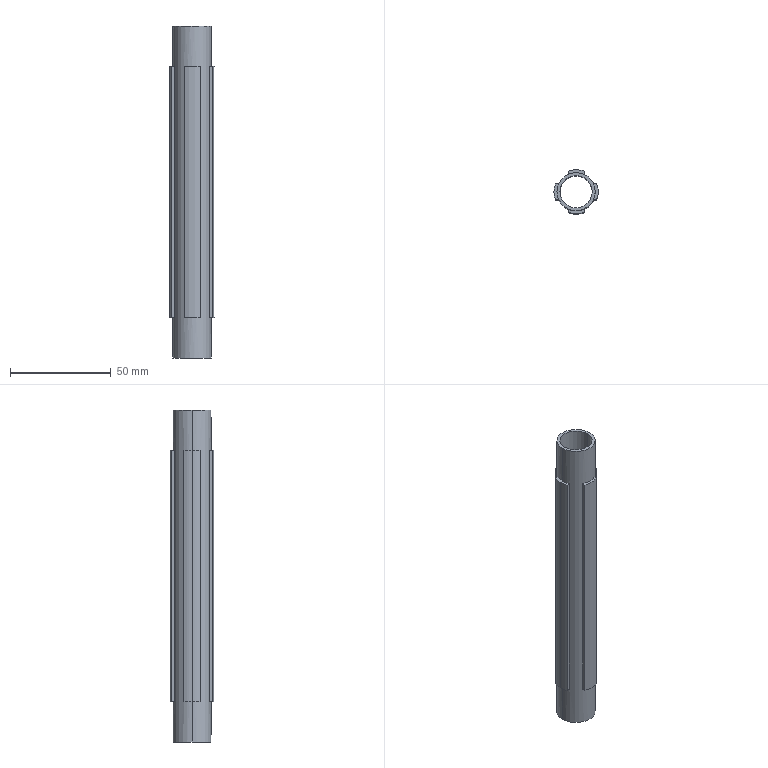Part | SolidWorks | features Extrusion 1, ICE 1 | 1 solid | 27 faces | box 22 x 22 x 165 mm | volume 19772 mm3 | plane 18 | cylinder 9 | commonest cylinder face diameters 22 x5 16 x2 19 x2
STEP:
#1=CARTESIAN_POINT('',(-8.,0.,145.));
#2=VERTEX_POINT('',#1);
#3=CARTESIAN_POINT('',(8.,0.,145.));
#4=VERTEX_POINT('',#3);
#5=CARTESIAN_POINT('',(0.,0.,145.));
#6=DIRECTION('',(0.,0.,1.));
#7=DIRECTION('',(1.,0.,0.));
#8=AXIS2_PLACEMENT_3D('',#5,#6,#7);
#9=CIRCLE('',#8,8.);
#10=EDGE_CURVE('',#2,#4,#9,.T.);
#11=ORIENTED_EDGE('',*,*,#10,.T.);
#12=CARTESIAN_POINT('',(8.,0.,-20.));
#13=VERTEX_POINT('',#12);
#14=CARTESIAN_POINT('',(8.,0.,125.));
#15=DIRECTION('',(0.,0.,-1.));
#16=VECTOR('',#15,1000.);
#17=LINE('',#14,#16);
#18=EDGE_CURVE('',#4,#13,#17,.T.);
#19=ORIENTED_EDGE('',*,*,#18,.T.);
#20=CARTESIAN_POINT('',(-8.,0.,-20.));
#21=VERTEX_POINT('',#20);
#22=CARTESIAN_POINT('',(0.,0.,-20.));
#23=DIRECTION('',(0.,0.,1.));
#24=DIRECTION('',(1.,0.,0.));
#25=AXIS2_PLACEMENT_3D('',#22,#23,#24);
#26=CIRCLE('',#25,8.);
#27=EDGE_CURVE('',#21,#13,#26,.T.);
#28=ORIENTED_EDGE('',*,*,#27,.F.);
#29=CARTESIAN_POINT('',(-8.,0.,125.));
#30=DIRECTION('',(0.,0.,-1.));
#31=VECTOR('',#30,1000.);
#32=LINE('',#29,#31);
#33=EDGE_CURVE('',#2,#21,#32,.T.);
#34=ORIENTED_EDGE('',*,*,#33,.F.);
#35=EDGE_LOOP('',(#11,#19,#28,#34));
#36=FACE_OUTER_BOUND('',#35,.T.);
#37=CARTESIAN_POINT('',(0.,0.,125.));
#38=DIRECTION('',(0.,0.,-1.));
#39=DIRECTION('',(-1.,0.,0.));
#40=AXIS2_PLACEMENT_3D('',#37,#38,#39);
#41=CYLINDRICAL_SURFACE('',#40,8.);
#42=ADVANCED_FACE('',(#36),#41,.F.);
#43=CARTESIAN_POINT('',(4.,8.617,125.));
#44=VERTEX_POINT('',#43);
#45=CARTESIAN_POINT('',(4.,8.617,0.));
#46=VERTEX_POINT('',#45);
#47=CARTESIAN_POINT('',(4.,8.617,125.));
#48=DIRECTION('',(0.,0.,-1.));
#49=VECTOR('',#48,1000.);
#50=LINE('',#47,#49);
#51=EDGE_CURVE('',#44,#46,#50,.T.);
#52=ORIENTED_EDGE('',*,*,#51,.F.);
#53=CARTESIAN_POINT('',(-4.,8.617,125.));
#54=VERTEX_POINT('',#53);
#55=CARTESIAN_POINT('',(0.,0.,125.));
#56=DIRECTION('',(0.,0.,1.));
#57=DIRECTION('',(1.,0.,0.));
#58=AXIS2_PLACEMENT_3D('',#55,#56,#57);
#59=CIRCLE('',#58,9.5);
#60=EDGE_CURVE('',#44,#54,#59,.T.);
#61=ORIENTED_EDGE('',*,*,#60,.T.);
#62=CARTESIAN_POINT('',(-4.,8.617,0.));
#63=VERTEX_POINT('',#62);
#64=CARTESIAN_POINT('',(-4.,8.617,125.));
#65=DIRECTION('',(0.,0.,-1.));
#66=VECTOR('',#65,1000.);
#67=LINE('',#64,#66);
#68=EDGE_CURVE('',#54,#63,#67,.T.);
#69=ORIENTED_EDGE('',*,*,#68,.T.);
#70=CARTESIAN_POINT('',(0.,0.,0.));
#71=DIRECTION('',(0.,0.,1.));
#72=DIRECTION('',(1.,0.,0.));
#73=AXIS2_PLACEMENT_3D('',#70,#71,#72);
#74=CIRCLE('',#73,9.5);
#75=EDGE_CURVE('',#46,#63,#74,.T.);
#76=ORIENTED_EDGE('',*,*,#75,.F.);
#77=EDGE_LOOP('',(#52,#61,#69,#76));
#78=FACE_BOUND('',#77,.T.);
#79=CARTESIAN_POINT('',(9.5,0.,145.));
#80=VERTEX_POINT('',#79);
#81=CARTESIAN_POINT('',(-9.5,0.,145.));
#82=VERTEX_POINT('',#81);
#83=CARTESIAN_POINT('',(0.,0.,145.));
#84=DIRECTION('',(0.,0.,1.));
#85=DIRECTION('',(1.,0.,0.));
#86=AXIS2_PLACEMENT_3D('',#83,#84,#85);
#87=CIRCLE('',#86,9.5);
#88=EDGE_CURVE('',#80,#82,#87,.T.);
#89=ORIENTED_EDGE('',*,*,#88,.F.);
#90=CARTESIAN_POINT('',(9.5,0.,125.));
#91=VERTEX_POINT('',#90);
#92=CARTESIAN_POINT('',(9.5,0.,125.));
#93=DIRECTION('',(0.,0.,-1.));
#94=VECTOR('',#93,1000.);
#95=LINE('',#92,#94);
#96=EDGE_CURVE('',#80,#91,#95,.T.);
#97=ORIENTED_EDGE('',*,*,#96,.T.);
#98=CARTESIAN_POINT('',(8.617,4.,125.));
#99=VERTEX_POINT('',#98);
#100=CARTESIAN_POINT('',(0.,0.,125.));
#101=DIRECTION('',(0.,0.,1.));
#102=DIRECTION('',(1.,0.,0.));
#103=AXIS2_PLACEMENT_3D('',#100,#101,#102);
#104=CIRCLE('',#103,9.5);
#105=EDGE_CURVE('',#91,#99,#104,.T.);
#106=ORIENTED_EDGE('',*,*,#105,.T.);
#107=CARTESIAN_POINT('',(8.617,4.,0.));
#108=VERTEX_POINT('',#107);
#109=CARTESIAN_POINT('',(8.617,4.,125.));
#110=DIRECTION('',(0.,0.,-1.));
#111=VECTOR('',#110,1000.);
#112=LINE('',#109,#111);
#113=EDGE_CURVE('',#99,#108,#112,.T.);
#114=ORIENTED_EDGE('',*,*,#113,.T.);
#115=CARTESIAN_POINT('',(9.5,0.,0.));
#116=VERTEX_POINT('',#115);
#117=CARTESIAN_POINT('',(0.,0.,0.));
#118=DIRECTION('',(0.,0.,1.));
#119=DIRECTION('',(1.,0.,0.));
#120=AXIS2_PLACEMENT_3D('',#117,#118,#119);
#121=CIRCLE('',#120,9.5);
#122=EDGE_CURVE('',#116,#108,#121,.T.);
#123=ORIENTED_EDGE('',*,*,#122,.F.);
#124=CARTESIAN_POINT('',(9.5,0.,-20.));
#125=VERTEX_POINT('',#124);
#126=CARTESIAN_POINT('',(9.5,0.,125.));
#127=DIRECTION('',(0.,0.,-1.));
#128=VECTOR('',#127,1000.);
#129=LINE('',#126,#128);
#130=EDGE_CURVE('',#116,#125,#129,.T.);
#131=ORIENTED_EDGE('',*,*,#130,.T.);
#132=CARTESIAN_POINT('',(-9.5,0.,-20.));
#133=VERTEX_POINT('',#132);
#134=CARTESIAN_POINT('',(0.,0.,-20.));
#135=DIRECTION('',(0.,0.,1.));
#136=DIRECTION('',(1.,0.,0.));
#137=AXIS2_PLACEMENT_3D('',#134,#135,#136);
#138=CIRCLE('',#137,9.5);
#139=EDGE_CURVE('',#125,#133,#138,.T.);
#140=ORIENTED_EDGE('',*,*,#139,.T.);
#141=CARTESIAN_POINT('',(-9.5,0.,0.));
#142=VERTEX_POINT('',#141);
#143=CARTESIAN_POINT('',(-9.5,0.,125.));
#144=DIRECTION('',(0.,0.,-1.));
#145=VECTOR('',#144,1000.);
#146=LINE('',#143,#145);
#147=EDGE_CURVE('',#142,#133,#146,.T.);
#148=ORIENTED_EDGE('',*,*,#147,.F.);
#149=CARTESIAN_POINT('',(-8.617,4.,0.));
#150=VERTEX_POINT('',#149);
#151=CARTESIAN_POINT('',(0.,0.,0.));
#152=DIRECTION('',(0.,0.,1.));
#153=DIRECTION('',(1.,0.,0.));
#154=AXIS2_PLACEMENT_3D('',#151,#152,#153);
#155=CIRCLE('',#154,9.5);
#156=EDGE_CURVE('',#150,#142,#155,.T.);
#157=ORIENTED_EDGE('',*,*,#156,.F.);
#158=CARTESIAN_POINT('',(-8.617,4.,125.));
#159=VERTEX_POINT('',#158);
#160=CARTESIAN_POINT('',(-8.617,4.,125.));
#161=DIRECTION('',(0.,0.,-1.));
#162=VECTOR('',#161,1000.);
#163=LINE('',#160,#162);
#164=EDGE_CURVE('',#159,#150,#163,.T.);
#165=ORIENTED_EDGE('',*,*,#164,.F.);
#166=CARTESIAN_POINT('',(-9.5,0.,125.));
#167=VERTEX_POINT('',#166);
#168=CARTESIAN_POINT('',(0.,0.,125.));
#169=DIRECTION('',(0.,0.,1.));
#170=DIRECTION('',(1.,0.,0.));
#171=AXIS2_PLACEMENT_3D('',#168,#169,#170);
#172=CIRCLE('',#171,9.5);
#173=EDGE_CURVE('',#159,#167,#172,.T.);
#174=ORIENTED_EDGE('',*,*,#173,.T.);
#175=CARTESIAN_POINT('',(-9.5,0.,125.));
#176=DIRECTION('',(0.,0.,-1.));
#177=VECTOR('',#176,1000.);
#178=LINE('',#175,#177);
#179=EDGE_CURVE('',#82,#167,#178,.T.);
#180=ORIENTED_EDGE('',*,*,#179,.F.);
#181=EDGE_LOOP('',(#89,#97,#106,#114,#123,#131,#140,#148,#157,#165,#174,#180));
#182=FACE_OUTER_BOUND('',#181,.T.);
#183=CARTESIAN_POINT('',(0.,0.,125.));
#184=DIRECTION('',(0.,0.,-1.));
#185=DIRECTION('',(-1.,0.,0.));
#186=AXIS2_PLACEMENT_3D('',#183,#184,#185);
#187=CYLINDRICAL_SURFACE('',#186,9.5);
#188=ADVANCED_FACE('',(#78,#182),#187,.T.);
#189=CARTESIAN_POINT('',(-11.,0.,125.));
#190=VERTEX_POINT('',#189);
#191=CARTESIAN_POINT('',(-10.247,-4.,125.));
#192=VERTEX_POINT('',#191);
#193=CARTESIAN_POINT('',(0.,0.,125.));
#194=DIRECTION('',(0.,0.,1.));
#195=DIRECTION('',(1.,0.,0.));
#196=AXIS2_PLACEMENT_3D('',#193,#194,#195);
#197=CIRCLE('',#196,11.);
#198=EDGE_CURVE('',#190,#192,#197,.T.);
#199=ORIENTED_EDGE('',*,*,#198,.F.);
#200=CARTESIAN_POINT('',(-11.,0.,0.));
#201=VERTEX_POINT('',#200);
#202=CARTESIAN_POINT('',(-11.,0.,125.));
#203=DIRECTION('',(0.,0.,-1.));
#204=VECTOR('',#203,1000.);
#205=LINE('',#202,#204);
#206=EDGE_CURVE('',#190,#201,#205,.T.);
#207=ORIENTED_EDGE('',*,*,#206,.T.);
#208=CARTESIAN_POINT('',(-10.247,-4.,0.));
#209=VERTEX_POINT('',#208);
#210=CARTESIAN_POINT('',(0.,0.,0.));
#211=DIRECTION('',(0.,0.,1.));
#212=DIRECTION('',(1.,0.,0.));
#213=AXIS2_PLACEMENT_3D('',#210,#211,#212);
#214=CIRCLE('',#213,11.);
#215=EDGE_CURVE('',#201,#209,#214,.T.);
#216=ORIENTED_EDGE('',*,*,#215,.T.);
#217=CARTESIAN_POINT('',(-10.247,-4.,125.));
#218=DIRECTION('',(0.,0.,-1.));
#219=VECTOR('',#218,1000.);
#220=LINE('',#217,#219);
#221=EDGE_CURVE('',#192,#209,#220,.T.);
#222=ORIENTED_EDGE('',*,*,#221,.F.);
#223=EDGE_LOOP('',(#199,#207,#216,#222));
#224=FACE_OUTER_BOUND('',#223,.T.);
#225=CARTESIAN_POINT('',(0.,0.,125.));
#226=DIRECTION('',(0.,0.,-1.));
#227=DIRECTION('',(-1.,0.,0.));
#228=AXIS2_PLACEMENT_3D('',#225,#226,#227);
#229=CYLINDRICAL_SURFACE('',#228,11.);
#230=ADVANCED_FACE('',(#224),#229,.T.);
#231=CARTESIAN_POINT('',(10.247,4.,125.));
#232=VERTEX_POINT('',#231);
#233=CARTESIAN_POINT('',(-0.0692,4.,125.));
#234=DIRECTION('',(-1.,0.,0.));
#235=VECTOR('',#234,1000.);
#236=LINE('',#233,#235);
#237=EDGE_CURVE('',#232,#99,#236,.T.);
#238=ORIENTED_EDGE('',*,*,#237,.T.);
#239=ORIENTED_EDGE('',*,*,#105,.F.);
#240=CARTESIAN_POINT('',(8.617,-4.,125.));
#241=VERTEX_POINT('',#240);
#242=CARTESIAN_POINT('',(0.,0.,125.));
#243=DIRECTION('',(0.,0.,1.));
#244=DIRECTION('',(1.,0.,0.));
#245=AXIS2_PLACEMENT_3D('',#242,#243,#244);
#246=CIRCLE('',#245,9.5);
#247=EDGE_CURVE('',#241,#91,#246,.T.);
#248=ORIENTED_EDGE('',*,*,#247,.F.);
#249=CARTESIAN_POINT('',(10.247,-4.,125.));
#250=VERTEX_POINT('',#249);
#251=CARTESIAN_POINT('',(-0.0692,-4.,125.));
#252=DIRECTION('',(-1.,0.,0.));
#253=VECTOR('',#252,1000.);
#254=LINE('',#251,#253);
#255=EDGE_CURVE('',#250,#241,#254,.T.);
#256=ORIENTED_EDGE('',*,*,#255,.F.);
#257=CARTESIAN_POINT('',(0.,0.,125.));
#258=DIRECTION('',(0.,0.,1.));
#259=DIRECTION('',(1.,0.,0.));
#260=AXIS2_PLACEMENT_3D('',#257,#258,#259);
#261=CIRCLE('',#260,11.);
#262=EDGE_CURVE('',#250,#232,#261,.T.);
#263=ORIENTED_EDGE('',*,*,#262,.T.);
#264=EDGE_LOOP('',(#238,#239,#248,#256,#263));
#265=FACE_OUTER_BOUND('',#264,.T.);
#266=CARTESIAN_POINT('',(-0.0692,-23.027,125.));
#267=DIRECTION('',(0.,0.,1.));
#268=DIRECTION('',(1.,0.,0.));
#269=AXIS2_PLACEMENT_3D('',#266,#267,#268);
#270=PLANE('',#269);
#271=ADVANCED_FACE('',(#265),#270,.T.);
#272=ORIENTED_EDGE('',*,*,#60,.F.);
#273=CARTESIAN_POINT('',(4.,10.247,125.));
#274=VERTEX_POINT('',#273);
#275=CARTESIAN_POINT('',(4.,-23.027,125.));
#276=DIRECTION('',(0.,-1.,0.));
#277=VECTOR('',#276,1000.);
#278=LINE('',#275,#277);
#279=EDGE_CURVE('',#274,#44,#278,.T.);
#280=ORIENTED_EDGE('',*,*,#279,.F.);
#281=CARTESIAN_POINT('',(-4.,10.247,125.));
#282=VERTEX_POINT('',#281);
#283=CARTESIAN_POINT('',(0.,0.,125.));
#284=DIRECTION('',(0.,0.,1.));
#285=DIRECTION('',(1.,0.,0.));
#286=AXIS2_PLACEMENT_3D('',#283,#284,#285);
#287=CIRCLE('',#286,11.);
#288=EDGE_CURVE('',#274,#282,#287,.T.);
#289=ORIENTED_EDGE('',*,*,#288,.T.);
#290=CARTESIAN_POINT('',(-4.,-23.027,125.));
#291=DIRECTION('',(0.,-1.,0.));
#292=VECTOR('',#291,1000.);
#293=LINE('',#290,#292);
#294=EDGE_CURVE('',#282,#54,#293,.T.);
#295=ORIENTED_EDGE('',*,*,#294,.T.);
#296=EDGE_LOOP('',(#272,#280,#289,#295));
#297=FACE_OUTER_BOUND('',#296,.T.);
#298=CARTESIAN_POINT('',(-0.0692,-23.027,125.));
#299=DIRECTION('',(0.,0.,1.));
#300=DIRECTION('',(1.,0.,0.));
#301=AXIS2_PLACEMENT_3D('',#298,#299,#300);
#302=PLANE('',#301);
#303=ADVANCED_FACE('',(#297),#302,.T.);
#304=ORIENTED_EDGE('',*,*,#173,.F.);
#305=CARTESIAN_POINT('',(-10.247,4.,125.));
#306=VERTEX_POINT('',#305);
#307=CARTESIAN_POINT('',(-0.0692,4.,125.));
#308=DIRECTION('',(1.,0.,0.));
#309=VECTOR('',#308,1000.);
#310=LINE('',#307,#309);
#311=EDGE_CURVE('',#306,#159,#310,.T.);
#312=ORIENTED_EDGE('',*,*,#311,.F.);
#313=CARTESIAN_POINT('',(0.,0.,125.));
#314=DIRECTION('',(0.,0.,1.));
#315=DIRECTION('',(1.,0.,0.));
#316=AXIS2_PLACEMENT_3D('',#313,#314,#315);
#317=CIRCLE('',#316,11.);
#318=EDGE_CURVE('',#306,#190,#317,.T.);
#319=ORIENTED_EDGE('',*,*,#318,.T.);
#320=ORIENTED_EDGE('',*,*,#198,.T.);
#321=CARTESIAN_POINT('',(-8.617,-4.,125.));
#322=VERTEX_POINT('',#321);
#323=CARTESIAN_POINT('',(-0.0692,-4.,125.));
#324=DIRECTION('',(1.,0.,0.));
#325=VECTOR('',#324,1000.);
#326=LINE('',#323,#325);
#327=EDGE_CURVE('',#192,#322,#326,.T.);
#328=ORIENTED_EDGE('',*,*,#327,.T.);
#329=CARTESIAN_POINT('',(0.,0.,125.));
#330=DIRECTION('',(0.,0.,1.));
#331=DIRECTION('',(1.,0.,0.));
#332=AXIS2_PLACEMENT_3D('',#329,#330,#331);
#333=CIRCLE('',#332,9.5);
#334=EDGE_CURVE('',#167,#322,#333,.T.);
#335=ORIENTED_EDGE('',*,*,#334,.F.);
#336=EDGE_LOOP('',(#304,#312,#319,#320,#328,#335));
#337=FACE_OUTER_BOUND('',#336,.T.);
#338=CARTESIAN_POINT('',(-0.0692,-23.027,125.));
#339=DIRECTION('',(0.,0.,1.));
#340=DIRECTION('',(1.,0.,0.));
#341=AXIS2_PLACEMENT_3D('',#338,#339,#340);
#342=PLANE('',#341);
#343=ADVANCED_FACE('',(#337),#342,.T.);
#344=CARTESIAN_POINT('',(8.617,-4.,0.));
#345=VERTEX_POINT('',#344);
#346=CARTESIAN_POINT('',(0.,0.,0.));
#347=DIRECTION('',(0.,0.,1.));
#348=DIRECTION('',(1.,0.,0.));
#349=AXIS2_PLACEMENT_3D('',#346,#347,#348);
#350=CIRCLE('',#349,9.5);
#351=EDGE_CURVE('',#345,#116,#350,.T.);
#352=ORIENTED_EDGE('',*,*,#351,.T.);
#353=ORIENTED_EDGE('',*,*,#122,.T.);
#354=CARTESIAN_POINT('',(10.247,4.,0.));
#355=VERTEX_POINT('',#354);
#356=CARTESIAN_POINT('',(-0.0692,4.,0.));
#357=DIRECTION('',(-1.,0.,0.));
#358=VECTOR('',#357,1000.);
#359=LINE('',#356,#358);
#360=EDGE_CURVE('',#355,#108,#359,.T.);
#361=ORIENTED_EDGE('',*,*,#360,.F.);
#362=CARTESIAN_POINT('',(10.247,-4.,0.));
#363=VERTEX_POINT('',#362);
#364=CARTESIAN_POINT('',(0.,0.,0.));
#365=DIRECTION('',(0.,0.,1.));
#366=DIRECTION('',(1.,0.,0.));
#367=AXIS2_PLACEMENT_3D('',#364,#365,#366);
#368=CIRCLE('',#367,11.);
#369=EDGE_CURVE('',#363,#355,#368,.T.);
#370=ORIENTED_EDGE('',*,*,#369,.F.);
#371=CARTESIAN_POINT('',(-0.0692,-4.,0.));
#372=DIRECTION('',(-1.,0.,0.));
#373=VECTOR('',#372,1000.);
#374=LINE('',#371,#373);
#375=EDGE_CURVE('',#363,#345,#374,.T.);
#376=ORIENTED_EDGE('',*,*,#375,.T.);
#377=EDGE_LOOP('',(#352,#353,#361,#370,#376));
#378=FACE_OUTER_BOUND('',#377,.T.);
#379=CARTESIAN_POINT('',(-0.0692,-23.027,0.));
#380=DIRECTION('',(0.,0.,1.));
#381=DIRECTION('',(1.,0.,0.));
#382=AXIS2_PLACEMENT_3D('',#379,#380,#381);
#383=PLANE('',#382);
#384=ADVANCED_FACE('',(#378),#383,.F.);
#385=CARTESIAN_POINT('',(4.,10.247,0.));
#386=VERTEX_POINT('',#385);
#387=CARTESIAN_POINT('',(4.,-23.027,0.));
#388=DIRECTION('',(0.,-1.,0.));
#389=VECTOR('',#388,1000.);
#390=LINE('',#387,#389);
#391=EDGE_CURVE('',#386,#46,#390,.T.);
#392=ORIENTED_EDGE('',*,*,#391,.T.);
#393=ORIENTED_EDGE('',*,*,#75,.T.);
#394=CARTESIAN_POINT('',(-4.,10.247,0.));
#395=VERTEX_POINT('',#394);
#396=CARTESIAN_POINT('',(-4.,-23.027,0.));
#397=DIRECTION('',(0.,-1.,0.));
#398=VECTOR('',#397,1000.);
#399=LINE('',#396,#398);
#400=EDGE_CURVE('',#395,#63,#399,.T.);
#401=ORIENTED_EDGE('',*,*,#400,.F.);
#402=CARTESIAN_POINT('',(0.,0.,0.));
#403=DIRECTION('',(0.,0.,1.));
#404=DIRECTION('',(1.,0.,0.));
#405=AXIS2_PLACEMENT_3D('',#402,#403,#404);
#406=CIRCLE('',#405,11.);
#407=EDGE_CURVE('',#386,#395,#406,.T.);
#408=ORIENTED_EDGE('',*,*,#407,.F.);
#409=EDGE_LOOP('',(#392,#393,#401,#408));
#410=FACE_OUTER_BOUND('',#409,.T.);
#411=CARTESIAN_POINT('',(-0.0692,-23.027,0.));
#412=DIRECTION('',(0.,0.,1.));
#413=DIRECTION('',(1.,0.,0.));
#414=AXIS2_PLACEMENT_3D('',#411,#412,#413);
#415=PLANE('',#414);
#416=ADVANCED_FACE('',(#410),#415,.F.);
#417=CARTESIAN_POINT('',(-10.247,4.,0.));
#418=VERTEX_POINT('',#417);
#419=CARTESIAN_POINT('',(-0.0692,4.,0.));
#420=DIRECTION('',(1.,0.,0.));
#421=VECTOR('',#420,1000.);
#422=LINE('',#419,#421);
#423=EDGE_CURVE('',#418,#150,#422,.T.);
#424=ORIENTED_EDGE('',*,*,#423,.T.);
#425=ORIENTED_EDGE('',*,*,#156,.T.);
#426=CARTESIAN_POINT('',(-8.617,-4.,0.));
#427=VERTEX_POINT('',#426);
#428=CARTESIAN_POINT('',(0.,0.,0.));
#429=DIRECTION('',(0.,0.,1.));
#430=DIRECTION('',(1.,0.,0.));
#431=AXIS2_PLACEMENT_3D('',#428,#429,#430);
#432=CIRCLE('',#431,9.5);
#433=EDGE_CURVE('',#142,#427,#432,.T.);
#434=ORIENTED_EDGE('',*,*,#433,.T.);
#435=CARTESIAN_POINT('',(-0.0692,-4.,0.));
#436=DIRECTION('',(1.,0.,0.));
#437=VECTOR('',#436,1000.);
#438=LINE('',#435,#437);
#439=EDGE_CURVE('',#209,#427,#438,.T.);
#440=ORIENTED_EDGE('',*,*,#439,.F.);
#441=ORIENTED_EDGE('',*,*,#215,.F.);
#442=CARTESIAN_POINT('',(0.,0.,0.));
#443=DIRECTION('',(0.,0.,1.));
#444=DIRECTION('',(1.,0.,0.));
#445=AXIS2_PLACEMENT_3D('',#442,#443,#444);
#446=CIRCLE('',#445,11.);
#447=EDGE_CURVE('',#418,#201,#446,.T.);
#448=ORIENTED_EDGE('',*,*,#447,.F.);
#449=EDGE_LOOP('',(#424,#425,#434,#440,#441,#448));
#450=FACE_OUTER_BOUND('',#449,.T.);
#451=CARTESIAN_POINT('',(-0.0692,-23.027,0.));
#452=DIRECTION('',(0.,0.,1.));
#453=DIRECTION('',(1.,0.,0.));
#454=AXIS2_PLACEMENT_3D('',#451,#452,#453);
#455=PLANE('',#454);
#456=ADVANCED_FACE('',(#450),#455,.F.);
#457=ORIENTED_EDGE('',*,*,#391,.F.);
#458=CARTESIAN_POINT('',(4.,10.247,125.));
#459=DIRECTION('',(0.,0.,-1.));
#460=VECTOR('',#459,1000.);
#461=LINE('',#458,#460);
#462=EDGE_CURVE('',#274,#386,#461,.T.);
#463=ORIENTED_EDGE('',*,*,#462,.F.);
#464=ORIENTED_EDGE('',*,*,#279,.T.);
#465=ORIENTED_EDGE('',*,*,#51,.T.);
#466=EDGE_LOOP('',(#457,#463,#464,#465));
#467=FACE_OUTER_BOUND('',#466,.T.);
#468=CARTESIAN_POINT('',(4.,-23.027,125.));
#469=DIRECTION('',(1.,0.,0.));
#470=DIRECTION('',(0.,0.,-1.));
#471=AXIS2_PLACEMENT_3D('',#468,#469,#470);
#472=PLANE('',#471);
#473=ADVANCED_FACE('',(#467),#472,.T.);
#474=ORIENTED_EDGE('',*,*,#407,.T.);
#475=CARTESIAN_POINT('',(-4.,10.247,125.));
#476=DIRECTION('',(0.,0.,-1.));
#477=VECTOR('',#476,1000.);
#478=LINE('',#475,#477);
#479=EDGE_CURVE('',#282,#395,#478,.T.);
#480=ORIENTED_EDGE('',*,*,#479,.F.);
#481=ORIENTED_EDGE('',*,*,#288,.F.);
#482=ORIENTED_EDGE('',*,*,#462,.T.);
#483=EDGE_LOOP('',(#474,#480,#481,#482));
#484=FACE_OUTER_BOUND('',#483,.T.);
#485=CARTESIAN_POINT('',(0.,0.,125.));
#486=DIRECTION('',(0.,0.,-1.));
#487=DIRECTION('',(-1.,0.,0.));
#488=AXIS2_PLACEMENT_3D('',#485,#486,#487);
#489=CYLINDRICAL_SURFACE('',#488,11.);
#490=ADVANCED_FACE('',(#484),#489,.T.);
#491=ORIENTED_EDGE('',*,*,#400,.T.);
#492=ORIENTED_EDGE('',*,*,#68,.F.);
#493=ORIENTED_EDGE('',*,*,#294,.F.);
#494=ORIENTED_EDGE('',*,*,#479,.T.);
#495=EDGE_LOOP('',(#491,#492,#493,#494));
#496=FACE_OUTER_BOUND('',#495,.T.);
#497=CARTESIAN_POINT('',(-4.,-23.027,125.));
#498=DIRECTION('',(1.,0.,0.));
#499=DIRECTION('',(0.,0.,-1.));
#500=AXIS2_PLACEMENT_3D('',#497,#498,#499);
#501=PLANE('',#500);
#502=ADVANCED_FACE('',(#496),#501,.F.);
#503=ORIENTED_EDGE('',*,*,#423,.F.);
#504=CARTESIAN_POINT('',(-10.247,4.,125.));
#505=DIRECTION('',(0.,0.,-1.));
#506=VECTOR('',#505,1000.);
#507=LINE('',#504,#506);
#508=EDGE_CURVE('',#306,#418,#507,.T.);
#509=ORIENTED_EDGE('',*,*,#508,.F.);
#510=ORIENTED_EDGE('',*,*,#311,.T.);
#511=ORIENTED_EDGE('',*,*,#164,.T.);
#512=EDGE_LOOP('',(#503,#509,#510,#511));
#513=FACE_OUTER_BOUND('',#512,.T.);
#514=CARTESIAN_POINT('',(-0.0692,4.,125.));
#515=DIRECTION('',(0.,1.,0.));
#516=DIRECTION('',(0.,0.,1.));
#517=AXIS2_PLACEMENT_3D('',#514,#515,#516);
#518=PLANE('',#517);
#519=ADVANCED_FACE('',(#513),#518,.T.);
#520=ORIENTED_EDGE('',*,*,#206,.F.);
#521=ORIENTED_EDGE('',*,*,#318,.F.);
#522=ORIENTED_EDGE('',*,*,#508,.T.);
#523=ORIENTED_EDGE('',*,*,#447,.T.);
#524=EDGE_LOOP('',(#520,#521,#522,#523));
#525=FACE_OUTER_BOUND('',#524,.T.);
#526=CARTESIAN_POINT('',(0.,0.,125.));
#527=DIRECTION('',(0.,0.,-1.));
#528=DIRECTION('',(-1.,0.,0.));
#529=AXIS2_PLACEMENT_3D('',#526,#527,#528);
#530=CYLINDRICAL_SURFACE('',#529,11.);
#531=ADVANCED_FACE('',(#525),#530,.T.);
#532=ORIENTED_EDGE('',*,*,#439,.T.);
#533=CARTESIAN_POINT('',(-8.617,-4.,125.));
#534=DIRECTION('',(0.,0.,-1.));
#535=VECTOR('',#534,1000.);
#536=LINE('',#533,#535);
#537=EDGE_CURVE('',#322,#427,#536,.T.);
#538=ORIENTED_EDGE('',*,*,#537,.F.);
#539=ORIENTED_EDGE('',*,*,#327,.F.);
#540=ORIENTED_EDGE('',*,*,#221,.T.);
#541=EDGE_LOOP('',(#532,#538,#539,#540));
#542=FACE_OUTER_BOUND('',#541,.T.);
#543=CARTESIAN_POINT('',(-0.0692,-4.,125.));
#544=DIRECTION('',(0.,1.,0.));
#545=DIRECTION('',(0.,0.,1.));
#546=AXIS2_PLACEMENT_3D('',#543,#544,#545);
#547=PLANE('',#546);
#548=ADVANCED_FACE('',(#542),#547,.F.);
#549=CARTESIAN_POINT('',(-4.,-10.247,0.));
#550=VERTEX_POINT('',#549);
#551=CARTESIAN_POINT('',(-4.,-8.617,0.));
#552=VERTEX_POINT('',#551);
#553=CARTESIAN_POINT('',(-4.,-23.027,0.));
#554=DIRECTION('',(0.,1.,0.));
#555=VECTOR('',#554,1000.);
#556=LINE('',#553,#555);
#557=EDGE_CURVE('',#550,#552,#556,.T.);
#558=ORIENTED_EDGE('',*,*,#557,.F.);
#559=CARTESIAN_POINT('',(-4.,-10.247,125.));
#560=VERTEX_POINT('',#559);
#561=CARTESIAN_POINT('',(-4.,-10.247,125.));
#562=DIRECTION('',(0.,0.,-1.));
#563=VECTOR('',#562,1000.);
#564=LINE('',#561,#563);
#565=EDGE_CURVE('',#560,#550,#564,.T.);
#566=ORIENTED_EDGE('',*,*,#565,.F.);
#567=CARTESIAN_POINT('',(-4.,-8.617,125.));
#568=VERTEX_POINT('',#567);
#569=CARTESIAN_POINT('',(-4.,-23.027,125.));
#570=DIRECTION('',(0.,1.,0.));
#571=VECTOR('',#570,1000.);
#572=LINE('',#569,#571);
#573=EDGE_CURVE('',#560,#568,#572,.T.);
#574=ORIENTED_EDGE('',*,*,#573,.T.);
#575=CARTESIAN_POINT('',(-4.,-8.617,125.));
#576=DIRECTION('',(0.,0.,-1.));
#577=VECTOR('',#576,1000.);
#578=LINE('',#575,#577);
#579=EDGE_CURVE('',#568,#552,#578,.T.);
#580=ORIENTED_EDGE('',*,*,#579,.T.);
#581=EDGE_LOOP('',(#558,#566,#574,#580));
#582=FACE_OUTER_BOUND('',#581,.T.);
#583=CARTESIAN_POINT('',(-4.,-23.027,125.));
#584=DIRECTION('',(-1.,0.,0.));
#585=DIRECTION('',(0.,-1.,0.));
#586=AXIS2_PLACEMENT_3D('',#583,#584,#585);
#587=PLANE('',#586);
#588=ADVANCED_FACE('',(#582),#587,.T.);
#589=CARTESIAN_POINT('',(4.,-10.247,0.));
#590=VERTEX_POINT('',#589);
#591=CARTESIAN_POINT('',(0.,0.,0.));
#592=DIRECTION('',(0.,0.,1.));
#593=DIRECTION('',(1.,0.,0.));
#594=AXIS2_PLACEMENT_3D('',#591,#592,#593);
#595=CIRCLE('',#594,11.);
#596=EDGE_CURVE('',#550,#590,#595,.T.);
#597=ORIENTED_EDGE('',*,*,#596,.T.);
#598=CARTESIAN_POINT('',(4.,-10.247,125.));
#599=VERTEX_POINT('',#598);
#600=CARTESIAN_POINT('',(4.,-10.247,125.));
#601=DIRECTION('',(0.,0.,-1.));
#602=VECTOR('',#601,1000.);
#603=LINE('',#600,#602);
#604=EDGE_CURVE('',#599,#590,#603,.T.);
#605=ORIENTED_EDGE('',*,*,#604,.F.);
#606=CARTESIAN_POINT('',(0.,0.,125.));
#607=DIRECTION('',(0.,0.,1.));
#608=DIRECTION('',(1.,0.,0.));
#609=AXIS2_PLACEMENT_3D('',#606,#607,#608);
#610=CIRCLE('',#609,11.);
#611=EDGE_CURVE('',#560,#599,#610,.T.);
#612=ORIENTED_EDGE('',*,*,#611,.F.);
#613=ORIENTED_EDGE('',*,*,#565,.T.);
#614=EDGE_LOOP('',(#597,#605,#612,#613));
#615=FACE_OUTER_BOUND('',#614,.T.);
#616=CARTESIAN_POINT('',(0.,0.,125.));
#617=DIRECTION('',(0.,0.,-1.));
#618=DIRECTION('',(-1.,0.,0.));
#619=AXIS2_PLACEMENT_3D('',#616,#617,#618);
#620=CYLINDRICAL_SURFACE('',#619,11.);
#621=ADVANCED_FACE('',(#615),#620,.T.);
#622=CARTESIAN_POINT('',(4.,-8.617,0.));
#623=VERTEX_POINT('',#622);
#624=CARTESIAN_POINT('',(4.,-23.027,0.));
#625=DIRECTION('',(0.,1.,0.));
#626=VECTOR('',#625,1000.);
#627=LINE('',#624,#626);
#628=EDGE_CURVE('',#590,#623,#627,.T.);
#629=ORIENTED_EDGE('',*,*,#628,.T.);
#630=CARTESIAN_POINT('',(4.,-8.617,125.));
#631=VERTEX_POINT('',#630);
#632=CARTESIAN_POINT('',(4.,-8.617,125.));
#633=DIRECTION('',(0.,0.,-1.));
#634=VECTOR('',#633,1000.);
#635=LINE('',#632,#634);
#636=EDGE_CURVE('',#631,#623,#635,.T.);
#637=ORIENTED_EDGE('',*,*,#636,.F.);
#638=CARTESIAN_POINT('',(4.,-23.027,125.));
#639=DIRECTION('',(0.,1.,0.));
#640=VECTOR('',#639,1000.);
#641=LINE('',#638,#640);
#642=EDGE_CURVE('',#599,#631,#641,.T.);
#643=ORIENTED_EDGE('',*,*,#642,.F.);
#644=ORIENTED_EDGE('',*,*,#604,.T.);
#645=EDGE_LOOP('',(#629,#637,#643,#644));
#646=FACE_OUTER_BOUND('',#645,.T.);
#647=CARTESIAN_POINT('',(4.,-23.027,125.));
#648=DIRECTION('',(-1.,0.,0.));
#649=DIRECTION('',(0.,0.,1.));
#650=AXIS2_PLACEMENT_3D('',#647,#648,#649);
#651=PLANE('',#650);
#652=ADVANCED_FACE('',(#646),#651,.F.);
#653=ORIENTED_EDGE('',*,*,#375,.F.);
#654=CARTESIAN_POINT('',(10.247,-4.,125.));
#655=DIRECTION('',(0.,0.,-1.));
#656=VECTOR('',#655,1000.);
#657=LINE('',#654,#656);
#658=EDGE_CURVE('',#250,#363,#657,.T.);
#659=ORIENTED_EDGE('',*,*,#658,.F.);
#660=ORIENTED_EDGE('',*,*,#255,.T.);
#661=CARTESIAN_POINT('',(8.617,-4.,125.));
#662=DIRECTION('',(0.,0.,-1.));
#663=VECTOR('',#662,1000.);
#664=LINE('',#661,#663);
#665=EDGE_CURVE('',#241,#345,#664,.T.);
#666=ORIENTED_EDGE('',*,*,#665,.T.);
#667=EDGE_LOOP('',(#653,#659,#660,#666));
#668=FACE_OUTER_BOUND('',#667,.T.);
#669=CARTESIAN_POINT('',(-0.0692,-4.,125.));
#670=DIRECTION('',(0.,-1.,0.));
#671=DIRECTION('',(0.,0.,-1.));
#672=AXIS2_PLACEMENT_3D('',#669,#670,#671);
#673=PLANE('',#672);
#674=ADVANCED_FACE('',(#668),#673,.T.);
#675=ORIENTED_EDGE('',*,*,#369,.T.);
#676=CARTESIAN_POINT('',(10.247,4.,125.));
#677=DIRECTION('',(0.,0.,-1.));
#678=VECTOR('',#677,1000.);
#679=LINE('',#676,#678);
#680=EDGE_CURVE('',#232,#355,#679,.T.);
#681=ORIENTED_EDGE('',*,*,#680,.F.);
#682=ORIENTED_EDGE('',*,*,#262,.F.);
#683=ORIENTED_EDGE('',*,*,#658,.T.);
#684=EDGE_LOOP('',(#675,#681,#682,#683));
#685=FACE_OUTER_BOUND('',#684,.T.);
#686=CARTESIAN_POINT('',(0.,0.,125.));
#687=DIRECTION('',(0.,0.,-1.));
#688=DIRECTION('',(-1.,0.,0.));
#689=AXIS2_PLACEMENT_3D('',#686,#687,#688);
#690=CYLINDRICAL_SURFACE('',#689,11.);
#691=ADVANCED_FACE('',(#685),#690,.T.);
#692=ORIENTED_EDGE('',*,*,#360,.T.);
#693=ORIENTED_EDGE('',*,*,#113,.F.);
#694=ORIENTED_EDGE('',*,*,#237,.F.);
#695=ORIENTED_EDGE('',*,*,#680,.T.);
#696=EDGE_LOOP('',(#692,#693,#694,#695));
#697=FACE_OUTER_BOUND('',#696,.T.);
#698=CARTESIAN_POINT('',(-0.0692,4.,125.));
#699=DIRECTION('',(0.,-1.,0.));
#700=DIRECTION('',(0.,0.,-1.));
#701=AXIS2_PLACEMENT_3D('',#698,#699,#700);
#702=PLANE('',#701);
#703=ADVANCED_FACE('',(#697),#702,.F.);
#704=ORIENTED_EDGE('',*,*,#96,.F.);
#705=CARTESIAN_POINT('',(0.,0.,145.));
#706=DIRECTION('',(0.,0.,1.));
#707=DIRECTION('',(1.,0.,0.));
#708=AXIS2_PLACEMENT_3D('',#705,#706,#707);
#709=CIRCLE('',#708,9.5);
#710=EDGE_CURVE('',#82,#80,#709,.T.);
#711=ORIENTED_EDGE('',*,*,#710,.F.);
#712=ORIENTED_EDGE('',*,*,#179,.T.);
#713=ORIENTED_EDGE('',*,*,#334,.T.);
#714=ORIENTED_EDGE('',*,*,#537,.T.);
#715=ORIENTED_EDGE('',*,*,#433,.F.);
#716=ORIENTED_EDGE('',*,*,#147,.T.);
#717=CARTESIAN_POINT('',(0.,0.,-20.));
#718=DIRECTION('',(0.,0.,1.));
#719=DIRECTION('',(1.,0.,0.));
#720=AXIS2_PLACEMENT_3D('',#717,#718,#719);
#721=CIRCLE('',#720,9.5);
#722=EDGE_CURVE('',#133,#125,#721,.T.);
#723=ORIENTED_EDGE('',*,*,#722,.T.);
#724=ORIENTED_EDGE('',*,*,#130,.F.);
#725=ORIENTED_EDGE('',*,*,#351,.F.);
#726=ORIENTED_EDGE('',*,*,#665,.F.);
#727=ORIENTED_EDGE('',*,*,#247,.T.);
#728=EDGE_LOOP('',(#704,#711,#712,#713,#714,#715,#716,#723,#724,#725,#726,#727));
#729=FACE_OUTER_BOUND('',#728,.T.);
#730=ORIENTED_EDGE('',*,*,#579,.F.);
#731=CARTESIAN_POINT('',(0.,0.,125.));
#732=DIRECTION('',(0.,0.,1.));
#733=DIRECTION('',(1.,0.,0.));
#734=AXIS2_PLACEMENT_3D('',#731,#732,#733);
#735=CIRCLE('',#734,9.5);
#736=EDGE_CURVE('',#568,#631,#735,.T.);
#737=ORIENTED_EDGE('',*,*,#736,.T.);
#738=ORIENTED_EDGE('',*,*,#636,.T.);
#739=CARTESIAN_POINT('',(0.,0.,0.));
#740=DIRECTION('',(0.,0.,1.));
#741=DIRECTION('',(1.,0.,0.));
#742=AXIS2_PLACEMENT_3D('',#739,#740,#741);
#743=CIRCLE('',#742,9.5);
#744=EDGE_CURVE('',#552,#623,#743,.T.);
#745=ORIENTED_EDGE('',*,*,#744,.F.);
#746=EDGE_LOOP('',(#730,#737,#738,#745));
#747=FACE_BOUND('',#746,.T.);
#748=CARTESIAN_POINT('',(0.,0.,125.));
#749=DIRECTION('',(0.,0.,-1.));
#750=DIRECTION('',(-1.,0.,0.));
#751=AXIS2_PLACEMENT_3D('',#748,#749,#750);
#752=CYLINDRICAL_SURFACE('',#751,9.5);
#753=ADVANCED_FACE('',(#729,#747),#752,.T.);
#754=ORIENTED_EDGE('',*,*,#736,.F.);
#755=ORIENTED_EDGE('',*,*,#573,.F.);
#756=ORIENTED_EDGE('',*,*,#611,.T.);
#757=ORIENTED_EDGE('',*,*,#642,.T.);
#758=EDGE_LOOP('',(#754,#755,#756,#757));
#759=FACE_OUTER_BOUND('',#758,.T.);
#760=CARTESIAN_POINT('',(-0.0692,-23.027,125.));
#761=DIRECTION('',(0.,0.,1.));
#762=DIRECTION('',(1.,0.,0.));
#763=AXIS2_PLACEMENT_3D('',#760,#761,#762);
#764=PLANE('',#763);
#765=ADVANCED_FACE('',(#759),#764,.T.);
#766=ORIENTED_EDGE('',*,*,#557,.T.);
#767=ORIENTED_EDGE('',*,*,#744,.T.);
#768=ORIENTED_EDGE('',*,*,#628,.F.);
#769=ORIENTED_EDGE('',*,*,#596,.F.);
#770=EDGE_LOOP('',(#766,#767,#768,#769));
#771=FACE_OUTER_BOUND('',#770,.T.);
#772=CARTESIAN_POINT('',(-0.0692,-23.027,0.));
#773=DIRECTION('',(0.,0.,1.));
#774=DIRECTION('',(1.,0.,0.));
#775=AXIS2_PLACEMENT_3D('',#772,#773,#774);
#776=PLANE('',#775);
#777=ADVANCED_FACE('',(#771),#776,.F.);
#778=ORIENTED_EDGE('',*,*,#27,.T.);
#779=CARTESIAN_POINT('',(0.,0.,-20.));
#780=DIRECTION('',(0.,0.,1.));
#781=DIRECTION('',(1.,0.,0.));
#782=AXIS2_PLACEMENT_3D('',#779,#780,#781);
#783=CIRCLE('',#782,8.);
#784=EDGE_CURVE('',#13,#21,#783,.T.);
#785=ORIENTED_EDGE('',*,*,#784,.T.);
#786=EDGE_LOOP('',(#778,#785));
#787=FACE_BOUND('',#786,.T.);
#788=ORIENTED_EDGE('',*,*,#722,.F.);
#789=ORIENTED_EDGE('',*,*,#139,.F.);
#790=EDGE_LOOP('',(#788,#789));
#791=FACE_OUTER_BOUND('',#790,.T.);
#792=CARTESIAN_POINT('',(0.,0.,-20.));
#793=DIRECTION('',(0.,0.,1.));
#794=DIRECTION('',(1.,0.,0.));
#795=AXIS2_PLACEMENT_3D('',#792,#793,#794);
#796=PLANE('',#795);
#797=ADVANCED_FACE('',(#787,#791),#796,.F.);
#798=ORIENTED_EDGE('',*,*,#710,.T.);
#799=ORIENTED_EDGE('',*,*,#88,.T.);
#800=EDGE_LOOP('',(#798,#799));
#801=FACE_OUTER_BOUND('',#800,.T.);
#802=ORIENTED_EDGE('',*,*,#10,.F.);
#803=CARTESIAN_POINT('',(0.,0.,145.));
#804=DIRECTION('',(0.,0.,1.));
#805=DIRECTION('',(1.,0.,0.));
#806=AXIS2_PLACEMENT_3D('',#803,#804,#805);
#807=CIRCLE('',#806,8.);
#808=EDGE_CURVE('',#4,#2,#807,.T.);
#809=ORIENTED_EDGE('',*,*,#808,.F.);
#810=EDGE_LOOP('',(#802,#809));
#811=FACE_BOUND('',#810,.T.);
#812=CARTESIAN_POINT('',(0.,0.,145.));
#813=DIRECTION('',(0.,0.,1.));
#814=DIRECTION('',(1.,0.,0.));
#815=AXIS2_PLACEMENT_3D('',#812,#813,#814);
#816=PLANE('',#815);
#817=ADVANCED_FACE('',(#801,#811),#816,.T.);
#818=ORIENTED_EDGE('',*,*,#18,.F.);
#819=ORIENTED_EDGE('',*,*,#808,.T.);
#820=ORIENTED_EDGE('',*,*,#33,.T.);
#821=ORIENTED_EDGE('',*,*,#784,.F.);
#822=EDGE_LOOP('',(#818,#819,#820,#821));
#823=FACE_OUTER_BOUND('',#822,.T.);
#824=CARTESIAN_POINT('',(0.,0.,125.));
#825=DIRECTION('',(0.,0.,-1.));
#826=DIRECTION('',(-1.,0.,0.));
#827=AXIS2_PLACEMENT_3D('',#824,#825,#826);
#828=CYLINDRICAL_SURFACE('',#827,8.);
#829=ADVANCED_FACE('',(#823),#828,.F.);
#830=CLOSED_SHELL('',(#42,#188,#230,#271,#303,#343,#384,#416,#456,#473,#490,#502,#519,#531,#548,#588,#621,#652,#674,#691,#703,#753,#765,#777,#797,#817,#829));
#831=MANIFOLD_SOLID_BREP('',#830);
#832=CARTESIAN_POINT('',(0.,0.,0.));
#833=DIRECTION('',(0.,0.,1.));
#834=DIRECTION('',(1.,0.,0.));
#835=AXIS2_PLACEMENT_3D('',#832,#833,#834);
#836=(LENGTH_UNIT()NAMED_UNIT(*)SI_UNIT(.MILLI.,.METRE.));
#837=UNCERTAINTY_MEASURE_WITH_UNIT(LENGTH_MEASURE(0.00001),#836,'','');
#838=(NAMED_UNIT(*)PLANE_ANGLE_UNIT()SI_UNIT($,.RADIAN.));
#839=(NAMED_UNIT(*)SI_UNIT($,.STERADIAN.)SOLID_ANGLE_UNIT());
#840=(GEOMETRIC_REPRESENTATION_CONTEXT(3)GLOBAL_UNCERTAINTY_ASSIGNED_CONTEXT((#837))GLOBAL_UNIT_ASSIGNED_CONTEXT((#836,#838,#839))REPRESENTATION_CONTEXT('',''));
#841=ADVANCED_BREP_SHAPE_REPRESENTATION('',(#831,#835),#840);